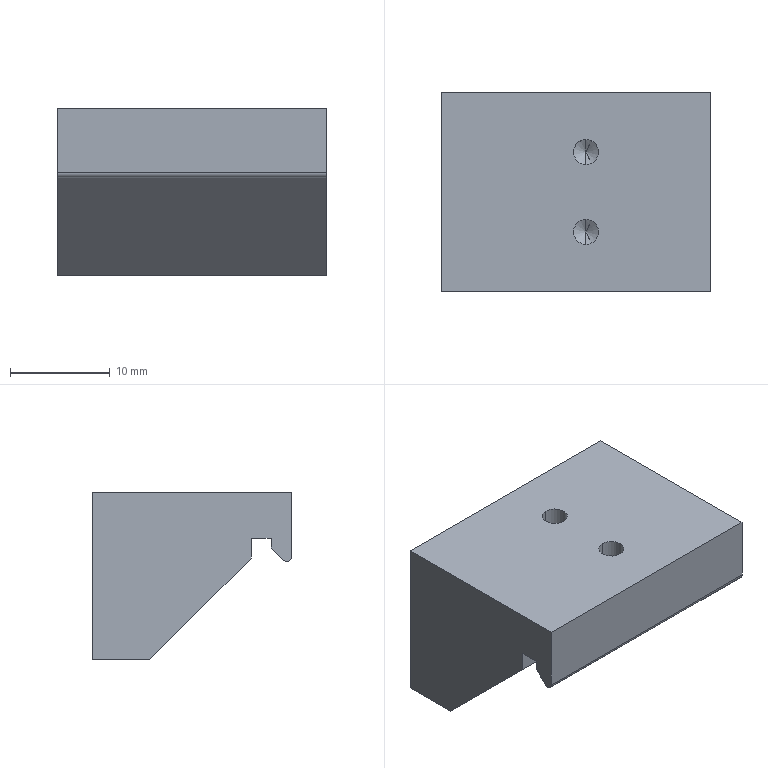CAM job | NX | 3-axis milling | part box 27 x 20 x 16.8 mm | stock box 31 x 24 x 17.8 mm
Tools:
number,name,description,diameter,corner_radius,flute_length,length,flutes
9,D10JING,Milling Tool-5 Parameters,10.0,0.0,50.0,75.0,2
10,D10,Milling Tool-5 Parameters,10.0,0.0,50.0,75.0,2
6,D6,Milling Tool-5 Parameters,6.0,0.0,50.0,75.0,2
2,D2,Milling Tool-5 Parameters,2.0,0.0,50.0,75.0,2
5,D2R0.5,Milling Tool-5 Parameters,2.0,0.5,50.0,75.0,2
7,D6A45,Milling Tool-5 Parameters,6.0,0.0,50.0,75.0,2
Operations:
program,operation,operation_type,tool,method,geometry_group,spindle_rpm,surface_speed,feed_per_tooth,feed_cut,feed_plunge,cut_length_mm,path_length_mm,cut_time_min,machine_time_min
1,FLOOR_WALL,VolumeBased25DMillingOperation,D10JING,METHOD,A,9500.0,298.0,0.0658,1250.0,100.0,236.997,290.997,0.1896,0.195
1,ZLEVEL_PROFILE,ZLevelMilling,D10,METHOD,A,9500.0,298.0,0.1316,2500.0,1000.0,4353.211,4426.86,1.764,1.772
1,CAVITY_MILL,CavityMilling,D10,METHOD,A,9500.0,298.0,0.1579,3000.0,1000.0,2692.733,3068.387,1.072,1.11
1,CAVITY_MILL_COPY,CavityMilling,D6,METHOD,A,9509.0,179.0,0.0789,1500.0,1000.0,88.657,312.278,0.0719,0.0942
1,CAVITY_MILL_COPY_COPY,CavityMilling,D2,METHOD,A,9974.0,94.0,0.0501,1000.0,1000.0,507.145,849.365,0.5071,0.5414
1,PLANAR_PROFILE,PlanarMilling,D2,METHOD,A,9500.0,59.0,0.0658,1250.0,100.0,574.0,652.4,0.4592,0.467
1,ZLEVEL_PROFILE_1,ZLevelMilling,D2R0.5,METHOD,A,9500.0,89.0,0.1316,2500.0,1000.0,5528.622,5593.378,2.214,2.22
1,ZLEVEL_PROFILE_1_COPY,ZLevelMilling,D2R0.5,METHOD,A,9500.0,89.0,0.1316,2500.0,1000.0,2079.903,2349.442,0.8383,0.8653
1,PLANAR_MILL_COPY_1,PlanarMilling,D6A45,METHOD,A,9500.0,179.0,0.0658,1250.0,100.0,46.372,105.372,0.0371,0.043
1,刀补9,ZLevelMilling,D10JING,METHOD,A,9500.0,298.0,0.0632,1200.0,1000.0,134.954,224.254,0.1132,0.1222